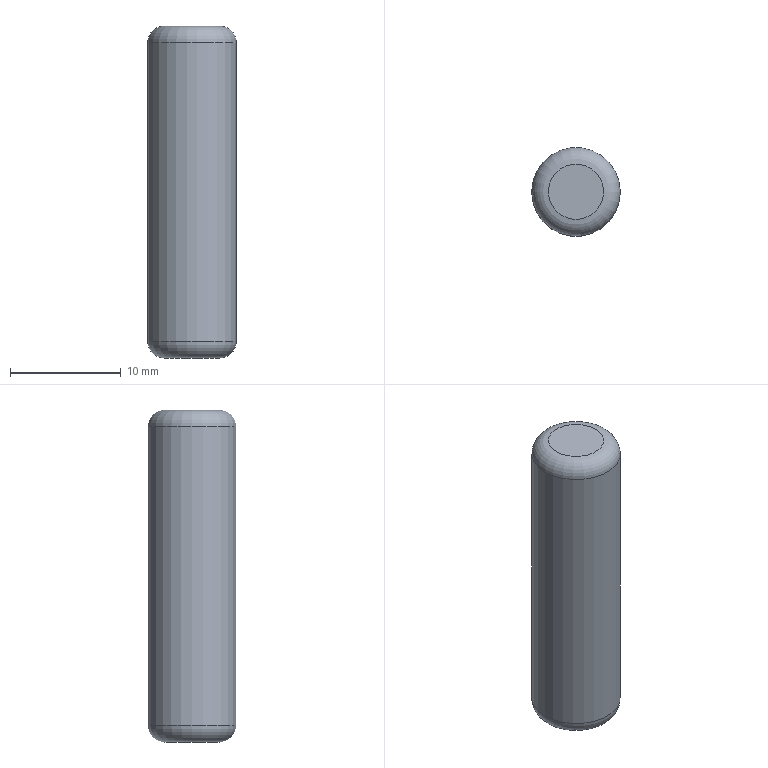Part | STEP file | 200 mesh_id742_x | 1 solid | 5 faces | box 8 x 8 x 30 mm | volume 1486 mm3 | plane 2 | torus 2 | cylinder 1 | commonest cylinder face diameters 8 x1
STEP:
#1=CARTESIAN_POINT('',(-17105.384,-4080.269,15.));
#2=VERTEX_POINT('',#1);
#3=CARTESIAN_POINT('',(-17107.884,-4080.269,15.));
#4=DIRECTION('',(0.,0.,1.));
#5=DIRECTION('',(1.,0.,0.));
#6=AXIS2_PLACEMENT_3D('',#3,#4,#5);
#7=CIRCLE('',#6,2.5);
#8=EDGE_CURVE('',#2,#2,#7,.T.);
#9=ORIENTED_EDGE('',*,*,#8,.T.);
#10=EDGE_LOOP('',(#9));
#11=FACE_OUTER_BOUND('',#10,.T.);
#12=CARTESIAN_POINT('',(-17107.884,-4080.269,15.));
#13=DIRECTION('',(0.,0.,1.));
#14=DIRECTION('',(1.,0.,0.));
#15=AXIS2_PLACEMENT_3D('',#12,#13,#14);
#16=PLANE('',#15);
#17=ADVANCED_FACE('',(#11),#16,.T.);
#18=CARTESIAN_POINT('',(-17110.384,-4080.269,-15.));
#19=VERTEX_POINT('',#18);
#20=CARTESIAN_POINT('',(-17107.884,-4080.269,-15.));
#21=DIRECTION('',(0.,0.,-1.));
#22=DIRECTION('',(-1.,0.,0.));
#23=AXIS2_PLACEMENT_3D('',#20,#21,#22);
#24=CIRCLE('',#23,2.5);
#25=EDGE_CURVE('',#19,#19,#24,.T.);
#26=ORIENTED_EDGE('',*,*,#25,.T.);
#27=EDGE_LOOP('',(#26));
#28=FACE_OUTER_BOUND('',#27,.T.);
#29=CARTESIAN_POINT('',(-17107.884,-4080.269,-15.));
#30=DIRECTION('',(0.,0.,-1.));
#31=DIRECTION('',(-1.,0.,0.));
#32=AXIS2_PLACEMENT_3D('',#29,#30,#31);
#33=PLANE('',#32);
#34=ADVANCED_FACE('',(#28),#33,.T.);
#35=CARTESIAN_POINT('',(-17111.884,-4080.269,-13.5));
#36=VERTEX_POINT('',#35);
#37=CARTESIAN_POINT('',(-17107.884,-4080.269,-13.5));
#38=DIRECTION('',(0.,0.,1.));
#39=DIRECTION('',(-1.,0.,0.));
#40=AXIS2_PLACEMENT_3D('',#37,#38,#39);
#41=CIRCLE('',#40,4.);
#42=EDGE_CURVE('',#36,#36,#41,.T.);
#43=ORIENTED_EDGE('',*,*,#42,.T.);
#44=EDGE_LOOP('',(#43));
#45=FACE_BOUND('',#44,.T.);
#46=CARTESIAN_POINT('',(-17103.884,-4080.269,13.5));
#47=VERTEX_POINT('',#46);
#48=CARTESIAN_POINT('',(-17107.884,-4080.269,13.5));
#49=DIRECTION('',(0.,0.,-1.));
#50=DIRECTION('',(1.,0.,0.));
#51=AXIS2_PLACEMENT_3D('',#48,#49,#50);
#52=CIRCLE('',#51,4.);
#53=EDGE_CURVE('',#47,#47,#52,.T.);
#54=ORIENTED_EDGE('',*,*,#53,.T.);
#55=EDGE_LOOP('',(#54));
#56=FACE_BOUND('',#55,.T.);
#57=CARTESIAN_POINT('',(-17107.884,-4080.269,0.));
#58=DIRECTION('',(0.,0.,1.));
#59=DIRECTION('',(1.,0.,0.));
#60=AXIS2_PLACEMENT_3D('',#57,#58,#59);
#61=CYLINDRICAL_SURFACE('',#60,4.);
#62=ADVANCED_FACE('',(#45,#56),#61,.T.);
#63=ORIENTED_EDGE('',*,*,#25,.F.);
#64=EDGE_LOOP('',(#63));
#65=FACE_BOUND('',#64,.T.);
#66=ORIENTED_EDGE('',*,*,#42,.F.);
#67=EDGE_LOOP('',(#66));
#68=FACE_BOUND('',#67,.T.);
#69=CARTESIAN_POINT('',(-17107.884,-4080.269,-13.5));
#70=DIRECTION('',(0.,0.,-1.));
#71=DIRECTION('',(-1.,0.,0.));
#72=AXIS2_PLACEMENT_3D('',#69,#70,#71);
#73=TOROIDAL_SURFACE('',#72,2.5,1.5);
#74=ADVANCED_FACE('',(#65,#68),#73,.T.);
#75=ORIENTED_EDGE('',*,*,#8,.F.);
#76=EDGE_LOOP('',(#75));
#77=FACE_BOUND('',#76,.T.);
#78=ORIENTED_EDGE('',*,*,#53,.F.);
#79=EDGE_LOOP('',(#78));
#80=FACE_BOUND('',#79,.T.);
#81=CARTESIAN_POINT('',(-17107.884,-4080.269,13.5));
#82=DIRECTION('',(0.,0.,1.));
#83=DIRECTION('',(1.,0.,0.));
#84=AXIS2_PLACEMENT_3D('',#81,#82,#83);
#85=TOROIDAL_SURFACE('',#84,2.5,1.5);
#86=ADVANCED_FACE('',(#77,#80),#85,.T.);
#87=CLOSED_SHELL('',(#17,#34,#62,#74,#86));
#88=MANIFOLD_SOLID_BREP('',#87);
#89=(LENGTH_UNIT()NAMED_UNIT(*)SI_UNIT(.MILLI.,.METRE.));
#90=UNCERTAINTY_MEASURE_WITH_UNIT(LENGTH_MEASURE(0.00002),#89,'','');
#91=(NAMED_UNIT(*)PLANE_ANGLE_UNIT()SI_UNIT($,.RADIAN.));
#92=PLANE_ANGLE_MEASURE_WITH_UNIT(PLANE_ANGLE_MEASURE(0.01745),#91);
#93=DIMENSIONAL_EXPONENTS(0.,0.,0.,0.,0.,0.,0.);
#94=(CONVERSION_BASED_UNIT('DEGREE',#92)NAMED_UNIT(#93)PLANE_ANGLE_UNIT());
#95=(NAMED_UNIT(*)SI_UNIT($,.STERADIAN.)SOLID_ANGLE_UNIT());
#96=(GEOMETRIC_REPRESENTATION_CONTEXT(3)GLOBAL_UNCERTAINTY_ASSIGNED_CONTEXT((#90))GLOBAL_UNIT_ASSIGNED_CONTEXT((#89,#94,#95))REPRESENTATION_CONTEXT('',''));
#97=ADVANCED_BREP_SHAPE_REPRESENTATION('',(#88),#96);